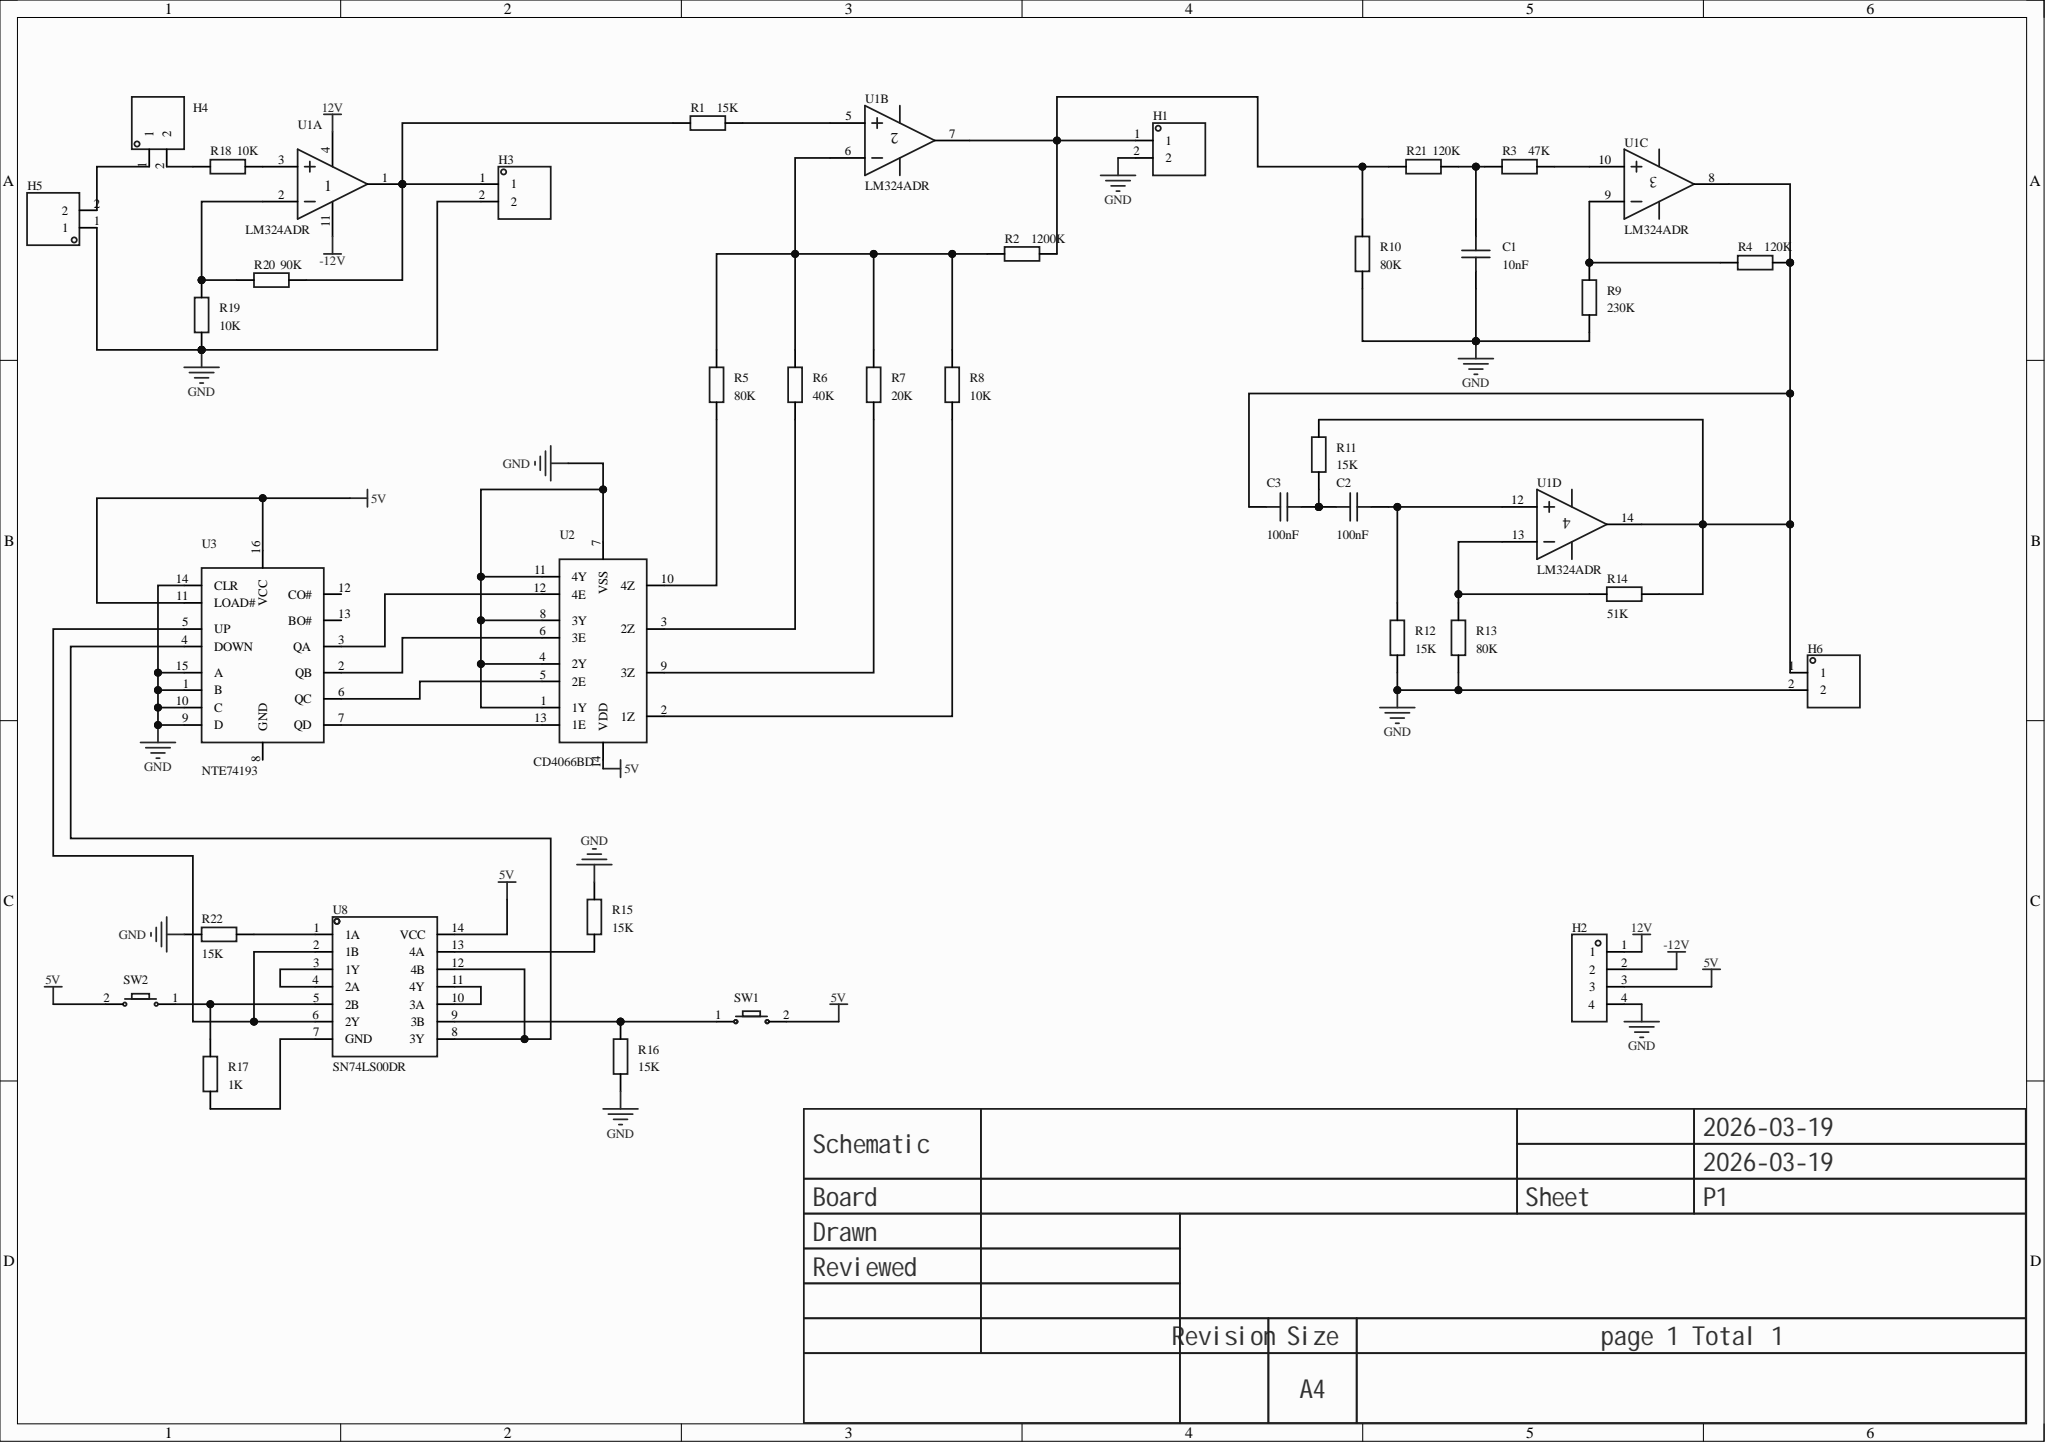Circuit board | Altium Designer | 37 parts | 36 nets
Bill of materials:
Comment,Description,Designator,Footprint,LibRef,Quantity
"10nF","","C1","CAP-TH_L5.0-W2.5-P5.00-D1.0","CAP_0603","1"
"100nF","","C2, C3","CAP-TH_L5.0-W2.5-P5.00-D1.0","CAP_0603","2"
"","","H1, H3, H4, H5, H6","HDR-TH_2P-P2.54-V-M-1","HDR-M_2.54_1x2P","5"
"","","H2","HDR-TH_4P-P2.54-V-M","HDR-M_2.54_1x4P","1"
"15K","","R1, R11, R12, R15, R16, R22","Res_1/8W","Res_0603","6"
"1200K","","R2","Res_1/8W","Res_0603","1"
"47K","","R3","Res_1/8W","Res_0603","1"
"120K","","R4, R21","Res_1/8W","Res_0603","2"
"80K","","R5, R10, R13","Res_1/8W","Res_0603","3"
"40K","","R6","Res_1/8W","Res_0603","1"
"20K","","R7","Res_1/8W","Res_0603","1"
"10K","","R8, R18, R19","Res_1/8W","Res_0603","3"
"230K","","R9","Res_1/8W","Res_0603","1"
"51K","","R14","Res_1/8W","Res_0603","1"
"1K","","R17","Res_1/8W","Res_0603","1"
"90K","","R20","Res_1/8W","Res_0603","1"
"","","SW1, SW2","Key_SMD_3x4x2","Key_SMD_3x4x2","2"
"LM324ADR","Amplifiers: quad; rail-to-rail: -; GBP: -; input offset voltage (Vos): 9mV; input bias current (Ib): 250nA;","U1","SOP-14_L8.6-W3.9-P1.27-LS6.0-BL","LM324ADR_C2837469","1"
"CD4066BD","Switch circuit: -; on-resistance (Ron): 1.05kO;","U2","SOP-14_L8.6-W3.9-P1.27-LS6.0-BL","CD4066BD","1"
"NTE74193","Operating voltage: -; component count: 1; count rate: 32MHz;","U3","PDIP-16_L19.7-W6.6-P2.54-LS7.6-BL","NTE74193","1"
"SN74LS00DR","Logic type: NAND gate; channels: 4; operating voltage: 4.75V~5.25V; propagation delay (tpd): 15ns@5V,15pF;","U8","SOIC-14_L8.7-W3.9-P1.27-LS6.0-BL","SN74LS00DR","1"
Netlist (Protel format):
[
C1
CAP-TH_L5.0-W2.5-P5.00-D1.0
10nF



]
[
C2
CAP-TH_L5.0-W2.5-P5.00-D1.0
100nF



]
[
C3
CAP-TH_L5.0-W2.5-P5.00-D1.0
100nF



]
[
H1
HDR-TH_2P-P2.54-V-M-1




]
[
H2
HDR-TH_4P-P2.54-V-M




]
[
H3
HDR-TH_2P-P2.54-V-M-1




]
[
H4
HDR-TH_2P-P2.54-V-M-1




]
[
H5
HDR-TH_2P-P2.54-V-M-1




]
[
H6
HDR-TH_2P-P2.54-V-M-1




]
[
R1
Res_1/8W
15K



]
[
R2
Res_1/8W
1200K



]
[
R3
Res_1/8W
47K



]
[
R4
Res_1/8W
120K



]
[
R5
Res_1/8W
80K



]
[
R6
Res_1/8W
40K



]
[
R7
Res_1/8W
20K



]
[
R8
Res_1/8W
10K



]
[
R9
Res_1/8W
230K



]
[
R10
Res_1/8W
80K



]
[
R11
Res_1/8W
15K



]
[
R12
Res_1/8W
15K



]
[
R13
Res_1/8W
80K



]
[
R14
Res_1/8W
51K



]
[
R15
Res_1/8W
15K



]
[
R16
Res_1/8W
15K



]
[
R17
Res_1/8W
1K



]
[
R18
Res_1/8W
10K



]
[
R19
Res_1/8W
10K



]
[
R20
Res_1/8W
90K



]
[
R21
Res_1/8W
120K



]
[
R22
Res_1/8W
15K



]
[
SW1
Key_SMD_3x4x2




]
[
SW2
Key_SMD_3x4x2




]
[
U1
SOP-14_L8.6-W3.9-P1.27-LS6.0-BL
LM324ADR



]
[
U2
SOP-14_L8.6-W3.9-P1.27-LS6.0-BL
CD4066BD



]
[
U3
PDIP-16_L19.7-W6.6-P2.54-LS7.6-BL
NTE74193



]
[
U8
SOIC-14_L8.7-W3.9-P1.27-LS6.0-BL
SN74LS00DR



]
(
NetU8_10
U8-10
U8-11
)
(
NetU8_3
U8-3
U8-4
)
(
NetU3_5
U3-5
U8-2
U8-6
)
(
NetU3_4
U3-4
U8-8
U8-12
)
(
NetU2_13
U2-13
U3-7
)
(
NetU2_12
U2-12
U3-3
)
(
NetU2_6
U2-6
U3-2
)
(
NetU2_5
U2-5
U3-6
)
(
NetR22_1
R22-1
U8-1
)
(
NetR19_2
R19-2
R20-1
U1-2
)
(
NetR18_2
R18-2
U1-3
)
(
NetR17_2
R17-2
SW2-1
U8-5
)
(
NetR17_1
R17-1
U8-7
)
(
NetR16_2
R16-2
SW1-1
U8-9
)
(
NetR15_1
R15-1
U8-13
)
(
NetR13_2
R13-2
R14-2
U1-13
)
(
NetR8_1
R8-1
U2-2
)
(
NetR7_1
R7-1
U2-9
)
(
NetR6_1
R6-1
U2-3
)
(
NetR5_1
R5-1
U2-10
)
(
NetR4_1
R4-1
R9-2
U1-9
)
(
NetR3_2
R3-2
U1-10
)
(
NetR2_1
R2-1
R5-2
R6-2
R7-2
R8-2
U1-6
)
(
NetR1_2
R1-2
U1-5
)
(
NetH4_2
H4-2
R18-1
)
(
NetH4_1
H4-1
H5-2
)
(
NetH3_1
H3-1
R1-1
R20-2
U1-1
)
(
NetH1_1
H1-1
R2-2
R10-2
R21-1
U1-7
)
(
NetC3_2
C3-2
H6-1
R4-2
R11-2
R14-1
U1-8
U1-14
)
(
NetC2_2
C2-2
C3-1
R11-1
)
(
NetC2_1
C2-1
R12-2
U1-12
)
(
NetC1_2
C1-2
R3-1
R21-2
)
(
GND
C1-1
H1-2
H2-4
H3-2
H5-1
H6-2
R9-1
R10-1
R12-1
R13-1
R15-2
R16-1
R19-1
R22-2
U2-1
U2-4
U2-7
U2-8
U2-11
U3-1
U3-9
U3-10
U3-14
U3-15
)
(
-12V
H2-2
U1-11
)
(
12V
H2-1
U1-4
)
(
5V
H2-3
SW1-2
SW2-2
U2-14
U3-11
U3-16
U8-14
)